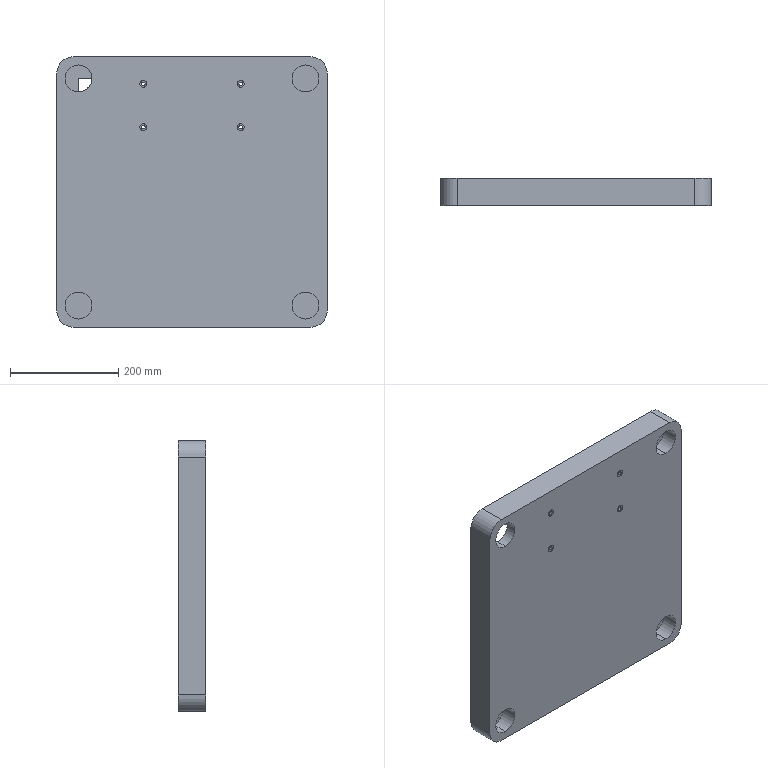Part | SolidWorks | features ICE 3, Extrusion 1, HoleWzd 1 | 1 solid | 50 faces | box 500 x 50 x 500 mm | volume 7022317 mm3 | cylinder 31 | plane 19 | commonest cylinder face diameters 6.6 x8 13 x8 50 x8 60 x4 70 x3
STEP:
#1=CARTESIAN_POINT('',(-90.,0.5,206.5));
#2=VERTEX_POINT('',#1);
#3=CARTESIAN_POINT('',(-90.,0.5,193.5));
#4=VERTEX_POINT('',#3);
#5=CARTESIAN_POINT('',(-90.,0.5,200.));
#6=DIRECTION('',(0.,-1.,0.));
#7=DIRECTION('',(0.,0.,-1.));
#8=AXIS2_PLACEMENT_3D('',#5,#6,#7);
#9=CIRCLE('',#8,6.5);
#10=EDGE_CURVE('',#2,#4,#9,.T.);
#11=ORIENTED_EDGE('',*,*,#10,.F.);
#12=CARTESIAN_POINT('',(-90.,0.,206.5));
#13=VERTEX_POINT('',#12);
#14=CARTESIAN_POINT('',(-90.,0.,206.5));
#15=DIRECTION('',(0.,-1.,0.));
#16=VECTOR('',#15,1000.);
#17=LINE('',#14,#16);
#18=EDGE_CURVE('',#2,#13,#17,.T.);
#19=ORIENTED_EDGE('',*,*,#18,.T.);
#20=CARTESIAN_POINT('',(-90.,0.,193.5));
#21=VERTEX_POINT('',#20);
#22=CARTESIAN_POINT('',(-90.,0.,200.));
#23=DIRECTION('',(0.,-1.,0.));
#24=DIRECTION('',(0.,0.,-1.));
#25=AXIS2_PLACEMENT_3D('',#22,#23,#24);
#26=CIRCLE('',#25,6.5);
#27=EDGE_CURVE('',#13,#21,#26,.T.);
#28=ORIENTED_EDGE('',*,*,#27,.T.);
#29=CARTESIAN_POINT('',(-90.,0.,193.5));
#30=DIRECTION('',(0.,-1.,0.));
#31=VECTOR('',#30,1000.);
#32=LINE('',#29,#31);
#33=EDGE_CURVE('',#4,#21,#32,.T.);
#34=ORIENTED_EDGE('',*,*,#33,.F.);
#35=EDGE_LOOP('',(#11,#19,#28,#34));
#36=FACE_OUTER_BOUND('',#35,.T.);
#37=CARTESIAN_POINT('',(-90.,0.,200.));
#38=DIRECTION('',(0.,-1.,0.));
#39=DIRECTION('',(0.,0.,-1.));
#40=AXIS2_PLACEMENT_3D('',#37,#38,#39);
#41=CYLINDRICAL_SURFACE('',#40,6.5);
#42=ADVANCED_FACE('',(#36),#41,.F.);
#43=CARTESIAN_POINT('',(-90.,20.,203.3));
#44=VERTEX_POINT('',#43);
#45=CARTESIAN_POINT('',(-90.,20.,196.7));
#46=VERTEX_POINT('',#45);
#47=CARTESIAN_POINT('',(-90.,20.,200.));
#48=DIRECTION('',(0.,-1.,0.));
#49=DIRECTION('',(0.,0.,-1.));
#50=AXIS2_PLACEMENT_3D('',#47,#48,#49);
#51=CIRCLE('',#50,3.3);
#52=EDGE_CURVE('',#44,#46,#51,.T.);
#53=ORIENTED_EDGE('',*,*,#52,.F.);
#54=CARTESIAN_POINT('',(-90.,0.5,203.3));
#55=VERTEX_POINT('',#54);
#56=CARTESIAN_POINT('',(-90.,0.,203.3));
#57=DIRECTION('',(0.,-1.,0.));
#58=VECTOR('',#57,1000.);
#59=LINE('',#56,#58);
#60=EDGE_CURVE('',#44,#55,#59,.T.);
#61=ORIENTED_EDGE('',*,*,#60,.T.);
#62=CARTESIAN_POINT('',(-90.,0.5,196.7));
#63=VERTEX_POINT('',#62);
#64=CARTESIAN_POINT('',(-90.,0.5,200.));
#65=DIRECTION('',(0.,-1.,0.));
#66=DIRECTION('',(0.,0.,-1.));
#67=AXIS2_PLACEMENT_3D('',#64,#65,#66);
#68=CIRCLE('',#67,3.3);
#69=EDGE_CURVE('',#55,#63,#68,.T.);
#70=ORIENTED_EDGE('',*,*,#69,.T.);
#71=CARTESIAN_POINT('',(-90.,0.,196.7));
#72=DIRECTION('',(0.,-1.,0.));
#73=VECTOR('',#72,1000.);
#74=LINE('',#71,#73);
#75=EDGE_CURVE('',#46,#63,#74,.T.);
#76=ORIENTED_EDGE('',*,*,#75,.F.);
#77=EDGE_LOOP('',(#53,#61,#70,#76));
#78=FACE_OUTER_BOUND('',#77,.T.);
#79=CARTESIAN_POINT('',(-90.,0.,200.));
#80=DIRECTION('',(0.,-1.,0.));
#81=DIRECTION('',(0.,0.,-1.));
#82=AXIS2_PLACEMENT_3D('',#79,#80,#81);
#83=CYLINDRICAL_SURFACE('',#82,3.3);
#84=ADVANCED_FACE('',(#78),#83,.F.);
#85=CARTESIAN_POINT('',(90.,0.5,126.5));
#86=VERTEX_POINT('',#85);
#87=CARTESIAN_POINT('',(90.,0.5,113.5));
#88=VERTEX_POINT('',#87);
#89=CARTESIAN_POINT('',(90.,0.5,120.));
#90=DIRECTION('',(0.,-1.,0.));
#91=DIRECTION('',(0.,0.,-1.));
#92=AXIS2_PLACEMENT_3D('',#89,#90,#91);
#93=CIRCLE('',#92,6.5);
#94=EDGE_CURVE('',#86,#88,#93,.T.);
#95=ORIENTED_EDGE('',*,*,#94,.F.);
#96=CARTESIAN_POINT('',(90.,0.,126.5));
#97=VERTEX_POINT('',#96);
#98=CARTESIAN_POINT('',(90.,0.,126.5));
#99=DIRECTION('',(0.,-1.,0.));
#100=VECTOR('',#99,1000.);
#101=LINE('',#98,#100);
#102=EDGE_CURVE('',#86,#97,#101,.T.);
#103=ORIENTED_EDGE('',*,*,#102,.T.);
#104=CARTESIAN_POINT('',(90.,0.,113.5));
#105=VERTEX_POINT('',#104);
#106=CARTESIAN_POINT('',(90.,0.,120.));
#107=DIRECTION('',(0.,-1.,0.));
#108=DIRECTION('',(0.,0.,-1.));
#109=AXIS2_PLACEMENT_3D('',#106,#107,#108);
#110=CIRCLE('',#109,6.5);
#111=EDGE_CURVE('',#97,#105,#110,.T.);
#112=ORIENTED_EDGE('',*,*,#111,.T.);
#113=CARTESIAN_POINT('',(90.,0.,113.5));
#114=DIRECTION('',(0.,-1.,0.));
#115=VECTOR('',#114,1000.);
#116=LINE('',#113,#115);
#117=EDGE_CURVE('',#88,#105,#116,.T.);
#118=ORIENTED_EDGE('',*,*,#117,.F.);
#119=EDGE_LOOP('',(#95,#103,#112,#118));
#120=FACE_OUTER_BOUND('',#119,.T.);
#121=CARTESIAN_POINT('',(90.,0.,120.));
#122=DIRECTION('',(0.,-1.,0.));
#123=DIRECTION('',(0.,0.,-1.));
#124=AXIS2_PLACEMENT_3D('',#121,#122,#123);
#125=CYLINDRICAL_SURFACE('',#124,6.5);
#126=ADVANCED_FACE('',(#120),#125,.F.);
#127=CARTESIAN_POINT('',(90.,20.,123.3));
#128=VERTEX_POINT('',#127);
#129=CARTESIAN_POINT('',(90.,20.,116.7));
#130=VERTEX_POINT('',#129);
#131=CARTESIAN_POINT('',(90.,20.,120.));
#132=DIRECTION('',(0.,-1.,0.));
#133=DIRECTION('',(0.,0.,-1.));
#134=AXIS2_PLACEMENT_3D('',#131,#132,#133);
#135=CIRCLE('',#134,3.3);
#136=EDGE_CURVE('',#128,#130,#135,.T.);
#137=ORIENTED_EDGE('',*,*,#136,.F.);
#138=CARTESIAN_POINT('',(90.,0.5,123.3));
#139=VERTEX_POINT('',#138);
#140=CARTESIAN_POINT('',(90.,0.,123.3));
#141=DIRECTION('',(0.,-1.,0.));
#142=VECTOR('',#141,1000.);
#143=LINE('',#140,#142);
#144=EDGE_CURVE('',#128,#139,#143,.T.);
#145=ORIENTED_EDGE('',*,*,#144,.T.);
#146=CARTESIAN_POINT('',(90.,0.5,116.7));
#147=VERTEX_POINT('',#146);
#148=CARTESIAN_POINT('',(90.,0.5,120.));
#149=DIRECTION('',(0.,-1.,0.));
#150=DIRECTION('',(0.,0.,-1.));
#151=AXIS2_PLACEMENT_3D('',#148,#149,#150);
#152=CIRCLE('',#151,3.3);
#153=EDGE_CURVE('',#139,#147,#152,.T.);
#154=ORIENTED_EDGE('',*,*,#153,.T.);
#155=CARTESIAN_POINT('',(90.,0.,116.7));
#156=DIRECTION('',(0.,-1.,0.));
#157=VECTOR('',#156,1000.);
#158=LINE('',#155,#157);
#159=EDGE_CURVE('',#130,#147,#158,.T.);
#160=ORIENTED_EDGE('',*,*,#159,.F.);
#161=EDGE_LOOP('',(#137,#145,#154,#160));
#162=FACE_OUTER_BOUND('',#161,.T.);
#163=CARTESIAN_POINT('',(90.,0.,120.));
#164=DIRECTION('',(0.,-1.,0.));
#165=DIRECTION('',(0.,0.,-1.));
#166=AXIS2_PLACEMENT_3D('',#163,#164,#165);
#167=CYLINDRICAL_SURFACE('',#166,3.3);
#168=ADVANCED_FACE('',(#162),#167,.F.);
#169=CARTESIAN_POINT('',(-90.,0.5,126.5));
#170=VERTEX_POINT('',#169);
#171=CARTESIAN_POINT('',(-90.,0.5,113.5));
#172=VERTEX_POINT('',#171);
#173=CARTESIAN_POINT('',(-90.,0.5,120.));
#174=DIRECTION('',(0.,-1.,0.));
#175=DIRECTION('',(0.,0.,-1.));
#176=AXIS2_PLACEMENT_3D('',#173,#174,#175);
#177=CIRCLE('',#176,6.5);
#178=EDGE_CURVE('',#170,#172,#177,.T.);
#179=ORIENTED_EDGE('',*,*,#178,.F.);
#180=CARTESIAN_POINT('',(-90.,0.,126.5));
#181=VERTEX_POINT('',#180);
#182=CARTESIAN_POINT('',(-90.,0.,126.5));
#183=DIRECTION('',(0.,-1.,0.));
#184=VECTOR('',#183,1000.);
#185=LINE('',#182,#184);
#186=EDGE_CURVE('',#170,#181,#185,.T.);
#187=ORIENTED_EDGE('',*,*,#186,.T.);
#188=CARTESIAN_POINT('',(-90.,0.,113.5));
#189=VERTEX_POINT('',#188);
#190=CARTESIAN_POINT('',(-90.,0.,120.));
#191=DIRECTION('',(0.,-1.,0.));
#192=DIRECTION('',(0.,0.,-1.));
#193=AXIS2_PLACEMENT_3D('',#190,#191,#192);
#194=CIRCLE('',#193,6.5);
#195=EDGE_CURVE('',#181,#189,#194,.T.);
#196=ORIENTED_EDGE('',*,*,#195,.T.);
#197=CARTESIAN_POINT('',(-90.,0.,113.5));
#198=DIRECTION('',(0.,-1.,0.));
#199=VECTOR('',#198,1000.);
#200=LINE('',#197,#199);
#201=EDGE_CURVE('',#172,#189,#200,.T.);
#202=ORIENTED_EDGE('',*,*,#201,.F.);
#203=EDGE_LOOP('',(#179,#187,#196,#202));
#204=FACE_OUTER_BOUND('',#203,.T.);
#205=CARTESIAN_POINT('',(-90.,0.,120.));
#206=DIRECTION('',(0.,-1.,0.));
#207=DIRECTION('',(0.,0.,-1.));
#208=AXIS2_PLACEMENT_3D('',#205,#206,#207);
#209=CYLINDRICAL_SURFACE('',#208,6.5);
#210=ADVANCED_FACE('',(#204),#209,.F.);
#211=CARTESIAN_POINT('',(-90.,20.,123.3));
#212=VERTEX_POINT('',#211);
#213=CARTESIAN_POINT('',(-90.,20.,116.7));
#214=VERTEX_POINT('',#213);
#215=CARTESIAN_POINT('',(-90.,20.,120.));
#216=DIRECTION('',(0.,-1.,0.));
#217=DIRECTION('',(0.,0.,-1.));
#218=AXIS2_PLACEMENT_3D('',#215,#216,#217);
#219=CIRCLE('',#218,3.3);
#220=EDGE_CURVE('',#212,#214,#219,.T.);
#221=ORIENTED_EDGE('',*,*,#220,.F.);
#222=CARTESIAN_POINT('',(-90.,0.5,123.3));
#223=VERTEX_POINT('',#222);
#224=CARTESIAN_POINT('',(-90.,0.,123.3));
#225=DIRECTION('',(0.,-1.,0.));
#226=VECTOR('',#225,1000.);
#227=LINE('',#224,#226);
#228=EDGE_CURVE('',#212,#223,#227,.T.);
#229=ORIENTED_EDGE('',*,*,#228,.T.);
#230=CARTESIAN_POINT('',(-90.,0.5,116.7));
#231=VERTEX_POINT('',#230);
#232=CARTESIAN_POINT('',(-90.,0.5,120.));
#233=DIRECTION('',(0.,-1.,0.));
#234=DIRECTION('',(0.,0.,-1.));
#235=AXIS2_PLACEMENT_3D('',#232,#233,#234);
#236=CIRCLE('',#235,3.3);
#237=EDGE_CURVE('',#223,#231,#236,.T.);
#238=ORIENTED_EDGE('',*,*,#237,.T.);
#239=CARTESIAN_POINT('',(-90.,0.,116.7));
#240=DIRECTION('',(0.,-1.,0.));
#241=VECTOR('',#240,1000.);
#242=LINE('',#239,#241);
#243=EDGE_CURVE('',#214,#231,#242,.T.);
#244=ORIENTED_EDGE('',*,*,#243,.F.);
#245=EDGE_LOOP('',(#221,#229,#238,#244));
#246=FACE_OUTER_BOUND('',#245,.T.);
#247=CARTESIAN_POINT('',(-90.,0.,120.));
#248=DIRECTION('',(0.,-1.,0.));
#249=DIRECTION('',(0.,0.,-1.));
#250=AXIS2_PLACEMENT_3D('',#247,#248,#249);
#251=CYLINDRICAL_SURFACE('',#250,3.3);
#252=ADVANCED_FACE('',(#246),#251,.F.);
#253=CARTESIAN_POINT('',(90.,0.5,206.5));
#254=VERTEX_POINT('',#253);
#255=CARTESIAN_POINT('',(90.,0.5,193.5));
#256=VERTEX_POINT('',#255);
#257=CARTESIAN_POINT('',(90.,0.5,200.));
#258=DIRECTION('',(0.,-1.,0.));
#259=DIRECTION('',(0.,0.,-1.));
#260=AXIS2_PLACEMENT_3D('',#257,#258,#259);
#261=CIRCLE('',#260,6.5);
#262=EDGE_CURVE('',#254,#256,#261,.T.);
#263=ORIENTED_EDGE('',*,*,#262,.F.);
#264=CARTESIAN_POINT('',(90.,0.,206.5));
#265=VERTEX_POINT('',#264);
#266=CARTESIAN_POINT('',(90.,0.,206.5));
#267=DIRECTION('',(0.,-1.,0.));
#268=VECTOR('',#267,1000.);
#269=LINE('',#266,#268);
#270=EDGE_CURVE('',#254,#265,#269,.T.);
#271=ORIENTED_EDGE('',*,*,#270,.T.);
#272=CARTESIAN_POINT('',(90.,0.,193.5));
#273=VERTEX_POINT('',#272);
#274=CARTESIAN_POINT('',(90.,0.,200.));
#275=DIRECTION('',(0.,-1.,0.));
#276=DIRECTION('',(0.,0.,-1.));
#277=AXIS2_PLACEMENT_3D('',#274,#275,#276);
#278=CIRCLE('',#277,6.5);
#279=EDGE_CURVE('',#265,#273,#278,.T.);
#280=ORIENTED_EDGE('',*,*,#279,.T.);
#281=CARTESIAN_POINT('',(90.,0.,193.5));
#282=DIRECTION('',(0.,-1.,0.));
#283=VECTOR('',#282,1000.);
#284=LINE('',#281,#283);
#285=EDGE_CURVE('',#256,#273,#284,.T.);
#286=ORIENTED_EDGE('',*,*,#285,.F.);
#287=EDGE_LOOP('',(#263,#271,#280,#286));
#288=FACE_OUTER_BOUND('',#287,.T.);
#289=CARTESIAN_POINT('',(90.,0.,200.));
#290=DIRECTION('',(0.,-1.,0.));
#291=DIRECTION('',(0.,0.,-1.));
#292=AXIS2_PLACEMENT_3D('',#289,#290,#291);
#293=CYLINDRICAL_SURFACE('',#292,6.5);
#294=ADVANCED_FACE('',(#288),#293,.F.);
#295=CARTESIAN_POINT('',(90.,20.,203.3));
#296=VERTEX_POINT('',#295);
#297=CARTESIAN_POINT('',(90.,20.,196.7));
#298=VERTEX_POINT('',#297);
#299=CARTESIAN_POINT('',(90.,20.,200.));
#300=DIRECTION('',(0.,-1.,0.));
#301=DIRECTION('',(0.,0.,-1.));
#302=AXIS2_PLACEMENT_3D('',#299,#300,#301);
#303=CIRCLE('',#302,3.3);
#304=EDGE_CURVE('',#296,#298,#303,.T.);
#305=ORIENTED_EDGE('',*,*,#304,.F.);
#306=CARTESIAN_POINT('',(90.,0.5,203.3));
#307=VERTEX_POINT('',#306);
#308=CARTESIAN_POINT('',(90.,0.,203.3));
#309=DIRECTION('',(0.,-1.,0.));
#310=VECTOR('',#309,1000.);
#311=LINE('',#308,#310);
#312=EDGE_CURVE('',#296,#307,#311,.T.);
#313=ORIENTED_EDGE('',*,*,#312,.T.);
#314=CARTESIAN_POINT('',(90.,0.5,196.7));
#315=VERTEX_POINT('',#314);
#316=CARTESIAN_POINT('',(90.,0.5,200.));
#317=DIRECTION('',(0.,-1.,0.));
#318=DIRECTION('',(0.,0.,-1.));
#319=AXIS2_PLACEMENT_3D('',#316,#317,#318);
#320=CIRCLE('',#319,3.3);
#321=EDGE_CURVE('',#307,#315,#320,.T.);
#322=ORIENTED_EDGE('',*,*,#321,.T.);
#323=CARTESIAN_POINT('',(90.,0.,196.7));
#324=DIRECTION('',(0.,-1.,0.));
#325=VECTOR('',#324,1000.);
#326=LINE('',#323,#325);
#327=EDGE_CURVE('',#298,#315,#326,.T.);
#328=ORIENTED_EDGE('',*,*,#327,.F.);
#329=EDGE_LOOP('',(#305,#313,#322,#328));
#330=FACE_OUTER_BOUND('',#329,.T.);
#331=CARTESIAN_POINT('',(90.,0.,200.));
#332=DIRECTION('',(0.,-1.,0.));
#333=DIRECTION('',(0.,0.,-1.));
#334=AXIS2_PLACEMENT_3D('',#331,#332,#333);
#335=CYLINDRICAL_SURFACE('',#334,3.3);
#336=ADVANCED_FACE('',(#330),#335,.F.);
#337=CARTESIAN_POINT('',(-210.,30.,-185.));
#338=VERTEX_POINT('',#337);
#339=CARTESIAN_POINT('',(-210.,30.,-235.));
#340=VERTEX_POINT('',#339);
#341=CARTESIAN_POINT('',(-210.,30.,-210.));
#342=DIRECTION('',(0.,-1.,0.));
#343=DIRECTION('',(0.,0.,1.));
#344=AXIS2_PLACEMENT_3D('',#341,#342,#343);
#345=CIRCLE('',#344,25.);
#346=EDGE_CURVE('',#338,#340,#345,.T.);
#347=ORIENTED_EDGE('',*,*,#346,.F.);
#348=CARTESIAN_POINT('',(-210.,0.,-185.));
#349=VERTEX_POINT('',#348);
#350=CARTESIAN_POINT('',(-210.,30.,-185.));
#351=DIRECTION('',(0.,-1.,0.));
#352=VECTOR('',#351,1000.);
#353=LINE('',#350,#352);
#354=EDGE_CURVE('',#338,#349,#353,.T.);
#355=ORIENTED_EDGE('',*,*,#354,.T.);
#356=CARTESIAN_POINT('',(-210.,0.,-235.));
#357=VERTEX_POINT('',#356);
#358=CARTESIAN_POINT('',(-210.,0.,-210.));
#359=DIRECTION('',(0.,-1.,0.));
#360=DIRECTION('',(0.,0.,1.));
#361=AXIS2_PLACEMENT_3D('',#358,#359,#360);
#362=CIRCLE('',#361,25.);
#363=EDGE_CURVE('',#349,#357,#362,.T.);
#364=ORIENTED_EDGE('',*,*,#363,.T.);
#365=CARTESIAN_POINT('',(-210.,30.,-235.));
#366=DIRECTION('',(0.,-1.,0.));
#367=VECTOR('',#366,1000.);
#368=LINE('',#365,#367);
#369=EDGE_CURVE('',#340,#357,#368,.T.);
#370=ORIENTED_EDGE('',*,*,#369,.F.);
#371=EDGE_LOOP('',(#347,#355,#364,#370));
#372=FACE_OUTER_BOUND('',#371,.T.);
#373=CARTESIAN_POINT('',(-210.,30.,-210.));
#374=DIRECTION('',(0.,-1.,0.));
#375=DIRECTION('',(0.,0.,-1.));
#376=AXIS2_PLACEMENT_3D('',#373,#374,#375);
#377=CYLINDRICAL_SURFACE('',#376,25.);
#378=ADVANCED_FACE('',(#372),#377,.F.);
#379=CARTESIAN_POINT('',(210.,30.,-185.));
#380=VERTEX_POINT('',#379);
#381=CARTESIAN_POINT('',(210.,30.,-235.));
#382=VERTEX_POINT('',#381);
#383=CARTESIAN_POINT('',(210.,30.,-210.));
#384=DIRECTION('',(0.,-1.,0.));
#385=DIRECTION('',(0.,0.,-1.));
#386=AXIS2_PLACEMENT_3D('',#383,#384,#385);
#387=CIRCLE('',#386,25.);
#388=EDGE_CURVE('',#380,#382,#387,.T.);
#389=ORIENTED_EDGE('',*,*,#388,.F.);
#390=CARTESIAN_POINT('',(210.,0.,-185.));
#391=VERTEX_POINT('',#390);
#392=CARTESIAN_POINT('',(210.,30.,-185.));
#393=DIRECTION('',(0.,-1.,0.));
#394=VECTOR('',#393,1000.);
#395=LINE('',#392,#394);
#396=EDGE_CURVE('',#380,#391,#395,.T.);
#397=ORIENTED_EDGE('',*,*,#396,.T.);
#398=CARTESIAN_POINT('',(210.,0.,-235.));
#399=VERTEX_POINT('',#398);
#400=CARTESIAN_POINT('',(210.,0.,-210.));
#401=DIRECTION('',(0.,-1.,0.));
#402=DIRECTION('',(0.,0.,-1.));
#403=AXIS2_PLACEMENT_3D('',#400,#401,#402);
#404=CIRCLE('',#403,25.);
#405=EDGE_CURVE('',#391,#399,#404,.T.);
#406=ORIENTED_EDGE('',*,*,#405,.T.);
#407=CARTESIAN_POINT('',(210.,30.,-235.));
#408=DIRECTION('',(0.,-1.,0.));
#409=VECTOR('',#408,1000.);
#410=LINE('',#407,#409);
#411=EDGE_CURVE('',#382,#399,#410,.T.);
#412=ORIENTED_EDGE('',*,*,#411,.F.);
#413=EDGE_LOOP('',(#389,#397,#406,#412));
#414=FACE_OUTER_BOUND('',#413,.T.);
#415=CARTESIAN_POINT('',(210.,30.,-210.));
#416=DIRECTION('',(0.,-1.,0.));
#417=DIRECTION('',(0.,0.,-1.));
#418=AXIS2_PLACEMENT_3D('',#415,#416,#417);
#419=CYLINDRICAL_SURFACE('',#418,25.);
#420=ADVANCED_FACE('',(#414),#419,.F.);
#421=CARTESIAN_POINT('',(210.,30.,235.));
#422=VERTEX_POINT('',#421);
#423=CARTESIAN_POINT('',(210.,30.,185.));
#424=VERTEX_POINT('',#423);
#425=CARTESIAN_POINT('',(210.,30.,210.));
#426=DIRECTION('',(0.,-1.,0.));
#427=DIRECTION('',(0.,0.,1.));
#428=AXIS2_PLACEMENT_3D('',#425,#426,#427);
#429=CIRCLE('',#428,25.);
#430=EDGE_CURVE('',#422,#424,#429,.T.);
#431=ORIENTED_EDGE('',*,*,#430,.F.);
#432=CARTESIAN_POINT('',(210.,0.,235.));
#433=VERTEX_POINT('',#432);
#434=CARTESIAN_POINT('',(210.,30.,235.));
#435=DIRECTION('',(0.,-1.,0.));
#436=VECTOR('',#435,1000.);
#437=LINE('',#434,#436);
#438=EDGE_CURVE('',#422,#433,#437,.T.);
#439=ORIENTED_EDGE('',*,*,#438,.T.);
#440=CARTESIAN_POINT('',(210.,0.,185.));
#441=VERTEX_POINT('',#440);
#442=CARTESIAN_POINT('',(210.,0.,210.));
#443=DIRECTION('',(0.,-1.,0.));
#444=DIRECTION('',(0.,0.,1.));
#445=AXIS2_PLACEMENT_3D('',#442,#443,#444);
#446=CIRCLE('',#445,25.);
#447=EDGE_CURVE('',#433,#441,#446,.T.);
#448=ORIENTED_EDGE('',*,*,#447,.T.);
#449=CARTESIAN_POINT('',(210.,30.,185.));
#450=DIRECTION('',(0.,-1.,0.));
#451=VECTOR('',#450,1000.);
#452=LINE('',#449,#451);
#453=EDGE_CURVE('',#424,#441,#452,.T.);
#454=ORIENTED_EDGE('',*,*,#453,.F.);
#455=EDGE_LOOP('',(#431,#439,#448,#454));
#456=FACE_OUTER_BOUND('',#455,.T.);
#457=CARTESIAN_POINT('',(210.,30.,210.));
#458=DIRECTION('',(0.,-1.,0.));
#459=DIRECTION('',(0.,0.,-1.));
#460=AXIS2_PLACEMENT_3D('',#457,#458,#459);
#461=CYLINDRICAL_SURFACE('',#460,25.);
#462=ADVANCED_FACE('',(#456),#461,.F.);
#463=CARTESIAN_POINT('',(-210.,30.,235.));
#464=VERTEX_POINT('',#463);
#465=CARTESIAN_POINT('',(-210.,30.,185.));
#466=VERTEX_POINT('',#465);
#467=CARTESIAN_POINT('',(-210.,30.,210.));
#468=DIRECTION('',(0.,-1.,0.));
#469=DIRECTION('',(0.,0.,-1.));
#470=AXIS2_PLACEMENT_3D('',#467,#468,#469);
#471=CIRCLE('',#470,25.);
#472=EDGE_CURVE('',#464,#466,#471,.T.);
#473=ORIENTED_EDGE('',*,*,#472,.F.);
#474=CARTESIAN_POINT('',(-210.,0.,235.));
#475=VERTEX_POINT('',#474);
#476=CARTESIAN_POINT('',(-210.,30.,235.));
#477=DIRECTION('',(0.,-1.,0.));
#478=VECTOR('',#477,1000.);
#479=LINE('',#476,#478);
#480=EDGE_CURVE('',#464,#475,#479,.T.);
#481=ORIENTED_EDGE('',*,*,#480,.T.);
#482=CARTESIAN_POINT('',(-210.,0.,185.));
#483=VERTEX_POINT('',#482);
#484=CARTESIAN_POINT('',(-210.,0.,210.));
#485=DIRECTION('',(0.,-1.,0.));
#486=DIRECTION('',(0.,0.,-1.));
#487=AXIS2_PLACEMENT_3D('',#484,#485,#486);
#488=CIRCLE('',#487,25.);
#489=EDGE_CURVE('',#475,#483,#488,.T.);
#490=ORIENTED_EDGE('',*,*,#489,.T.);
#491=CARTESIAN_POINT('',(-210.,20.,185.));
#492=VERTEX_POINT('',#491);
#493=CARTESIAN_POINT('',(-210.,30.,185.));
#494=DIRECTION('',(0.,-1.,0.));
#495=VECTOR('',#494,1000.);
#496=LINE('',#493,#495);
#497=EDGE_CURVE('',#492,#483,#496,.T.);
#498=ORIENTED_EDGE('',*,*,#497,.F.);
#499=CARTESIAN_POINT('',(-210.,30.,185.));
#500=DIRECTION('',(0.,1.,0.));
#501=VECTOR('',#500,1000.);
#502=LINE('',#499,#501);
#503=EDGE_CURVE('',#492,#466,#502,.T.);
#504=ORIENTED_EDGE('',*,*,#503,.T.);
#505=EDGE_LOOP('',(#473,#481,#490,#498,#504));
#506=FACE_OUTER_BOUND('',#505,.T.);
#507=CARTESIAN_POINT('',(-210.,30.,210.));
#508=DIRECTION('',(0.,-1.,0.));
#509=DIRECTION('',(0.,0.,-1.));
#510=AXIS2_PLACEMENT_3D('',#507,#508,#509);
#511=CYLINDRICAL_SURFACE('',#510,25.);
#512=ADVANCED_FACE('',(#506),#511,.F.);
#513=CARTESIAN_POINT('',(-250.,0.,220.));
#514=VERTEX_POINT('',#513);
#515=CARTESIAN_POINT('',(-220.,0.,250.));
#516=VERTEX_POINT('',#515);
#517=CARTESIAN_POINT('',(-220.,0.,220.));
#518=DIRECTION('',(0.,1.,0.));
#519=DIRECTION('',(0.,0.,-1.));
#520=AXIS2_PLACEMENT_3D('',#517,#518,#519);
#521=CIRCLE('',#520,30.);
#522=EDGE_CURVE('',#514,#516,#521,.T.);
#523=ORIENTED_EDGE('',*,*,#522,.T.);
#524=CARTESIAN_POINT('',(-220.,50.,250.));
#525=VERTEX_POINT('',#524);
#526=CARTESIAN_POINT('',(-220.,50.,250.));
#527=DIRECTION('',(0.,-1.,0.));
#528=VECTOR('',#527,1000.);
#529=LINE('',#526,#528);
#530=EDGE_CURVE('',#525,#516,#529,.T.);
#531=ORIENTED_EDGE('',*,*,#530,.F.);
#532=CARTESIAN_POINT('',(-250.,50.,220.));
#533=VERTEX_POINT('',#532);
#534=CARTESIAN_POINT('',(-220.,50.,220.));
#535=DIRECTION('',(0.,1.,0.));
#536=DIRECTION('',(0.,0.,-1.));
#537=AXIS2_PLACEMENT_3D('',#534,#535,#536);
#538=CIRCLE('',#537,30.);
#539=EDGE_CURVE('',#533,#525,#538,.T.);
#540=ORIENTED_EDGE('',*,*,#539,.F.);
#541=CARTESIAN_POINT('',(-250.,50.,220.));
#542=DIRECTION('',(0.,-1.,0.));
#543=VECTOR('',#542,1000.);
#544=LINE('',#541,#543);
#545=EDGE_CURVE('',#533,#514,#544,.T.);
#546=ORIENTED_EDGE('',*,*,#545,.T.);
#547=EDGE_LOOP('',(#523,#531,#540,#546));
#548=FACE_OUTER_BOUND('',#547,.T.);
#549=CARTESIAN_POINT('',(-220.,50.,220.));
#550=DIRECTION('',(0.,-1.,0.));
#551=DIRECTION('',(0.,0.,-1.));
#552=AXIS2_PLACEMENT_3D('',#549,#550,#551);
#553=CYLINDRICAL_SURFACE('',#552,30.);
#554=ADVANCED_FACE('',(#548),#553,.T.);
#555=CARTESIAN_POINT('',(220.,0.,250.));
#556=VERTEX_POINT('',#555);
#557=CARTESIAN_POINT('',(-220.,0.,250.));
#558=DIRECTION('',(1.,0.,0.));
#559=VECTOR('',#558,1000.);
#560=LINE('',#557,#559);
#561=EDGE_CURVE('',#516,#556,#560,.T.);
#562=ORIENTED_EDGE('',*,*,#561,.T.);
#563=CARTESIAN_POINT('',(220.,50.,250.));
#564=VERTEX_POINT('',#563);
#565=CARTESIAN_POINT('',(220.,50.,250.));
#566=DIRECTION('',(0.,-1.,0.));
#567=VECTOR('',#566,1000.);
#568=LINE('',#565,#567);
#569=EDGE_CURVE('',#564,#556,#568,.T.);
#570=ORIENTED_EDGE('',*,*,#569,.F.);
#571=CARTESIAN_POINT('',(-220.,50.,250.));
#572=DIRECTION('',(1.,0.,0.));
#573=VECTOR('',#572,1000.);
#574=LINE('',#571,#573);
#575=EDGE_CURVE('',#525,#564,#574,.T.);
#576=ORIENTED_EDGE('',*,*,#575,.F.);
#577=ORIENTED_EDGE('',*,*,#530,.T.);
#578=EDGE_LOOP('',(#562,#570,#576,#577));
#579=FACE_OUTER_BOUND('',#578,.T.);
#580=CARTESIAN_POINT('',(-220.,50.,250.));
#581=DIRECTION('',(0.,0.,-1.));
#582=DIRECTION('',(-1.,0.,0.));
#583=AXIS2_PLACEMENT_3D('',#580,#581,#582);
#584=PLANE('',#583);
#585=ADVANCED_FACE('',(#579),#584,.F.);
#586=CARTESIAN_POINT('',(250.,0.,220.));
#587=VERTEX_POINT('',#586);
#588=CARTESIAN_POINT('',(220.,0.,220.));
#589=DIRECTION('',(0.,1.,0.));
#590=DIRECTION('',(0.,0.,1.));
#591=AXIS2_PLACEMENT_3D('',#588,#589,#590);
#592=CIRCLE('',#591,30.);
#593=EDGE_CURVE('',#556,#587,#592,.T.);
#594=ORIENTED_EDGE('',*,*,#593,.T.);
#595=CARTESIAN_POINT('',(250.,50.,220.));
#596=VERTEX_POINT('',#595);
#597=CARTESIAN_POINT('',(250.,50.,220.));
#598=DIRECTION('',(0.,-1.,0.));
#599=VECTOR('',#598,1000.);
#600=LINE('',#597,#599);
#601=EDGE_CURVE('',#596,#587,#600,.T.);
#602=ORIENTED_EDGE('',*,*,#601,.F.);
#603=CARTESIAN_POINT('',(220.,50.,220.));
#604=DIRECTION('',(0.,1.,0.));
#605=DIRECTION('',(0.,0.,1.));
#606=AXIS2_PLACEMENT_3D('',#603,#604,#605);
#607=CIRCLE('',#606,30.);
#608=EDGE_CURVE('',#564,#596,#607,.T.);
#609=ORIENTED_EDGE('',*,*,#608,.F.);
#610=ORIENTED_EDGE('',*,*,#569,.T.);
#611=EDGE_LOOP('',(#594,#602,#609,#610));
#612=FACE_OUTER_BOUND('',#611,.T.);
#613=CARTESIAN_POINT('',(220.,50.,220.));
#614=DIRECTION('',(0.,-1.,0.));
#615=DIRECTION('',(0.,0.,-1.));
#616=AXIS2_PLACEMENT_3D('',#613,#614,#615);
#617=CYLINDRICAL_SURFACE('',#616,30.);
#618=ADVANCED_FACE('',(#612),#617,.T.);
#619=CARTESIAN_POINT('',(250.,0.,-220.));
#620=VERTEX_POINT('',#619);
#621=CARTESIAN_POINT('',(250.,0.,220.));
#622=DIRECTION('',(0.,0.,-1.));
#623=VECTOR('',#622,1000.);
#624=LINE('',#621,#623);
#625=EDGE_CURVE('',#587,#620,#624,.T.);
#626=ORIENTED_EDGE('',*,*,#625,.T.);
#627=CARTESIAN_POINT('',(250.,50.,-220.));
#628=VERTEX_POINT('',#627);
#629=CARTESIAN_POINT('',(250.,50.,-220.));
#630=DIRECTION('',(0.,-1.,0.));
#631=VECTOR('',#630,1000.);
#632=LINE('',#629,#631);
#633=EDGE_CURVE('',#628,#620,#632,.T.);
#634=ORIENTED_EDGE('',*,*,#633,.F.);
#635=CARTESIAN_POINT('',(250.,50.,220.));
#636=DIRECTION('',(0.,0.,-1.));
#637=VECTOR('',#636,1000.);
#638=LINE('',#635,#637);
#639=EDGE_CURVE('',#596,#628,#638,.T.);
#640=ORIENTED_EDGE('',*,*,#639,.F.);
#641=ORIENTED_EDGE('',*,*,#601,.T.);
#642=EDGE_LOOP('',(#626,#634,#640,#641));
#643=FACE_OUTER_BOUND('',#642,.T.);
#644=CARTESIAN_POINT('',(250.,50.,220.));
#645=DIRECTION('',(-1.,0.,0.));
#646=DIRECTION('',(0.,0.,1.));
#647=AXIS2_PLACEMENT_3D('',#644,#645,#646);
#648=PLANE('',#647);
#649=ADVANCED_FACE('',(#643),#648,.F.);
#650=CARTESIAN_POINT('',(220.,0.,-250.));
#651=VERTEX_POINT('',#650);
#652=CARTESIAN_POINT('',(220.,0.,-220.));
#653=DIRECTION('',(0.,1.,0.));
#654=DIRECTION('',(0.,0.,1.));
#655=AXIS2_PLACEMENT_3D('',#652,#653,#654);
#656=CIRCLE('',#655,30.);
#657=EDGE_CURVE('',#620,#651,#656,.T.);
#658=ORIENTED_EDGE('',*,*,#657,.T.);
#659=CARTESIAN_POINT('',(220.,50.,-250.));
#660=VERTEX_POINT('',#659);
#661=CARTESIAN_POINT('',(220.,50.,-250.));
#662=DIRECTION('',(0.,-1.,0.));
#663=VECTOR('',#662,1000.);
#664=LINE('',#661,#663);
#665=EDGE_CURVE('',#660,#651,#664,.T.);
#666=ORIENTED_EDGE('',*,*,#665,.F.);
#667=CARTESIAN_POINT('',(220.,50.,-220.));
#668=DIRECTION('',(0.,1.,0.));
#669=DIRECTION('',(0.,0.,1.));
#670=AXIS2_PLACEMENT_3D('',#667,#668,#669);
#671=CIRCLE('',#670,30.);
#672=EDGE_CURVE('',#628,#660,#671,.T.);
#673=ORIENTED_EDGE('',*,*,#672,.F.);
#674=ORIENTED_EDGE('',*,*,#633,.T.);
#675=EDGE_LOOP('',(#658,#666,#673,#674));
#676=FACE_OUTER_BOUND('',#675,.T.);
#677=CARTESIAN_POINT('',(220.,50.,-220.));
#678=DIRECTION('',(0.,-1.,0.));
#679=DIRECTION('',(0.,0.,-1.));
#680=AXIS2_PLACEMENT_3D('',#677,#678,#679);
#681=CYLINDRICAL_SURFACE('',#680,30.);
#682=ADVANCED_FACE('',(#676),#681,.T.);
#683=CARTESIAN_POINT('',(-220.,0.,-250.));
#684=VERTEX_POINT('',#683);
#685=CARTESIAN_POINT('',(-220.,0.,-250.));
#686=DIRECTION('',(-1.,0.,0.));
#687=VECTOR('',#686,1000.);
#688=LINE('',#685,#687);
#689=EDGE_CURVE('',#651,#684,#688,.T.);
#690=ORIENTED_EDGE('',*,*,#689,.T.);
#691=CARTESIAN_POINT('',(-220.,50.,-250.));
#692=VERTEX_POINT('',#691);
#693=CARTESIAN_POINT('',(-220.,50.,-250.));
#694=DIRECTION('',(0.,-1.,0.));
#695=VECTOR('',#694,1000.);
#696=LINE('',#693,#695);
#697=EDGE_CURVE('',#692,#684,#696,.T.);
#698=ORIENTED_EDGE('',*,*,#697,.F.);
#699=CARTESIAN_POINT('',(-220.,50.,-250.));
#700=DIRECTION('',(-1.,0.,0.));
#701=VECTOR('',#700,1000.);
#702=LINE('',#699,#701);
#703=EDGE_CURVE('',#660,#692,#702,.T.);
#704=ORIENTED_EDGE('',*,*,#703,.F.);
#705=ORIENTED_EDGE('',*,*,#665,.T.);
#706=EDGE_LOOP('',(#690,#698,#704,#705));
#707=FACE_OUTER_BOUND('',#706,.T.);
#708=CARTESIAN_POINT('',(-220.,50.,-250.));
#709=DIRECTION('',(0.,0.,1.));
#710=DIRECTION('',(1.,0.,0.));
#711=AXIS2_PLACEMENT_3D('',#708,#709,#710);
#712=PLANE('',#711);
#713=ADVANCED_FACE('',(#707),#712,.F.);
#714=CARTESIAN_POINT('',(-250.,0.,-220.));
#715=VERTEX_POINT('',#714);
#716=CARTESIAN_POINT('',(-220.,0.,-220.));
#717=DIRECTION('',(0.,1.,0.));
#718=DIRECTION('',(0.,0.,-1.));
#719=AXIS2_PLACEMENT_3D('',#716,#717,#718);
#720=CIRCLE('',#719,30.);
#721=EDGE_CURVE('',#684,#715,#720,.T.);
#722=ORIENTED_EDGE('',*,*,#721,.T.);
#723=CARTESIAN_POINT('',(-250.,50.,-220.));
#724=VERTEX_POINT('',#723);
#725=CARTESIAN_POINT('',(-250.,50.,-220.));
#726=DIRECTION('',(0.,-1.,0.));
#727=VECTOR('',#726,1000.);
#728=LINE('',#725,#727);
#729=EDGE_CURVE('',#724,#715,#728,.T.);
#730=ORIENTED_EDGE('',*,*,#729,.F.);
#731=CARTESIAN_POINT('',(-220.,50.,-220.));
#732=DIRECTION('',(0.,1.,0.));
#733=DIRECTION('',(0.,0.,-1.));
#734=AXIS2_PLACEMENT_3D('',#731,#732,#733);
#735=CIRCLE('',#734,30.);
#736=EDGE_CURVE('',#692,#724,#735,.T.);
#737=ORIENTED_EDGE('',*,*,#736,.F.);
#738=ORIENTED_EDGE('',*,*,#697,.T.);
#739=EDGE_LOOP('',(#722,#730,#737,#738));
#740=FACE_OUTER_BOUND('',#739,.T.);
#741=CARTESIAN_POINT('',(-220.,50.,-220.));
#742=DIRECTION('',(0.,-1.,0.));
#743=DIRECTION('',(0.,0.,-1.));
#744=AXIS2_PLACEMENT_3D('',#741,#742,#743);
#745=CYLINDRICAL_SURFACE('',#744,30.);
#746=ADVANCED_FACE('',(#740),#745,.T.);
#747=CARTESIAN_POINT('',(-250.,0.,220.));
#748=DIRECTION('',(0.,0.,1.));
#749=VECTOR('',#748,1000.);
#750=LINE('',#747,#749);
#751=EDGE_CURVE('',#715,#514,#750,.T.);
#752=ORIENTED_EDGE('',*,*,#751,.T.);
#753=ORIENTED_EDGE('',*,*,#545,.F.);
#754=CARTESIAN_POINT('',(-250.,50.,220.));
#755=DIRECTION('',(0.,0.,1.));
#756=VECTOR('',#755,1000.);
#757=LINE('',#754,#756);
#758=EDGE_CURVE('',#724,#533,#757,.T.);
#759=ORIENTED_EDGE('',*,*,#758,.F.);
#760=ORIENTED_EDGE('',*,*,#729,.T.);
#761=EDGE_LOOP('',(#752,#753,#759,#760));
#762=FACE_OUTER_BOUND('',#761,.T.);
#763=CARTESIAN_POINT('',(-250.,50.,220.));
#764=DIRECTION('',(1.,0.,0.));
#765=DIRECTION('',(0.,0.,-1.));
#766=AXIS2_PLACEMENT_3D('',#763,#764,#765);
#767=PLANE('',#766);
#768=ADVANCED_FACE('',(#762),#767,.F.);
#769=CARTESIAN_POINT('',(-210.,50.,210.));
#770=VERTEX_POINT('',#769);
#771=CARTESIAN_POINT('',(175.,50.,210.));
#772=VERTEX_POINT('',#771);
#773=CARTESIAN_POINT('',(-175.,50.,210.));
#774=DIRECTION('',(1.,0.,0.));
#775=VECTOR('',#774,1000.);
#776=LINE('',#773,#775);
#777=EDGE_CURVE('',#770,#772,#776,.T.);
#778=ORIENTED_EDGE('',*,*,#777,.F.);
#779=CARTESIAN_POINT('',(-210.,50.,-175.));
#780=VERTEX_POINT('',#779);
#781=CARTESIAN_POINT('',(-210.,50.,175.));
#782=DIRECTION('',(0.,0.,1.));
#783=VECTOR('',#782,1000.);
#784=LINE('',#781,#783);
#785=EDGE_CURVE('',#780,#770,#784,.T.);
#786=ORIENTED_EDGE('',*,*,#785,.F.);
#787=CARTESIAN_POINT('',(-175.,50.,-210.));
#788=VERTEX_POINT('',#787);
#789=CARTESIAN_POINT('',(-210.,50.,-210.));
#790=DIRECTION('',(0.,-1.,0.));
#791=DIRECTION('',(0.,0.,-1.));
#792=AXIS2_PLACEMENT_3D('',#789,#790,#791);
#793=CIRCLE('',#792,35.);
#794=EDGE_CURVE('',#788,#780,#793,.T.);
#795=ORIENTED_EDGE('',*,*,#794,.F.);
#796=CARTESIAN_POINT('',(175.,50.,-210.));
#797=VERTEX_POINT('',#796);
#798=CARTESIAN_POINT('',(-175.,50.,-210.));
#799=DIRECTION('',(-1.,0.,0.));
#800=VECTOR('',#799,1000.);
#801=LINE('',#798,#800);
#802=EDGE_CURVE('',#797,#788,#801,.T.);
#803=ORIENTED_EDGE('',*,*,#802,.F.);
#804=CARTESIAN_POINT('',(210.,50.,-175.));
#805=VERTEX_POINT('',#804);
#806=CARTESIAN_POINT('',(210.,50.,-210.));
#807=DIRECTION('',(0.,-1.,0.));
#808=DIRECTION('',(0.,0.,1.));
#809=AXIS2_PLACEMENT_3D('',#806,#807,#808);
#810=CIRCLE('',#809,35.);
#811=EDGE_CURVE('',#805,#797,#810,.T.);
#812=ORIENTED_EDGE('',*,*,#811,.F.);
#813=CARTESIAN_POINT('',(210.,50.,175.));
#814=VERTEX_POINT('',#813);
#815=CARTESIAN_POINT('',(210.,50.,175.));
#816=DIRECTION('',(0.,0.,-1.));
#817=VECTOR('',#816,1000.);
#818=LINE('',#815,#817);
#819=EDGE_CURVE('',#814,#805,#818,.T.);
#820=ORIENTED_EDGE('',*,*,#819,.F.);
#821=CARTESIAN_POINT('',(210.,50.,210.));
#822=DIRECTION('',(0.,-1.,0.));
#823=DIRECTION('',(0.,0.,-1.));
#824=AXIS2_PLACEMENT_3D('',#821,#822,#823);
#825=CIRCLE('',#824,35.);
#826=EDGE_CURVE('',#772,#814,#825,.T.);
#827=ORIENTED_EDGE('',*,*,#826,.F.);
#828=EDGE_LOOP('',(#778,#786,#795,#803,#812,#820,#827));
#829=FACE_BOUND('',#828,.T.);
#830=ORIENTED_EDGE('',*,*,#539,.T.);
#831=ORIENTED_EDGE('',*,*,#575,.T.);
#832=ORIENTED_EDGE('',*,*,#608,.T.);
#833=ORIENTED_EDGE('',*,*,#639,.T.);
#834=ORIENTED_EDGE('',*,*,#672,.T.);
#835=ORIENTED_EDGE('',*,*,#703,.T.);
#836=ORIENTED_EDGE('',*,*,#736,.T.);
#837=ORIENTED_EDGE('',*,*,#758,.T.);
#838=EDGE_LOOP('',(#830,#831,#832,#833,#834,#835,#836,#837));
#839=FACE_OUTER_BOUND('',#838,.T.);
#840=CARTESIAN_POINT('',(-220.,50.,220.));
#841=DIRECTION('',(0.,-1.,0.));
#842=DIRECTION('',(0.,0.,-1.));
#843=AXIS2_PLACEMENT_3D('',#840,#841,#842);
#844=PLANE('',#843);
#845=ADVANCED_FACE('',(#829,#839),#844,.F.);
#846=CARTESIAN_POINT('',(-90.,0.,200.));
#847=DIRECTION('',(0.,-1.,0.));
#848=DIRECTION('',(0.,0.,-1.));
#849=AXIS2_PLACEMENT_3D('',#846,#847,#848);
#850=CIRCLE('',#849,6.5);
#851=EDGE_CURVE('',#21,#13,#850,.T.);
#852=ORIENTED_EDGE('',*,*,#851,.F.);
#853=ORIENTED_EDGE('',*,*,#27,.F.);
#854=EDGE_LOOP('',(#852,#853));
#855=FACE_BOUND('',#854,.T.);
#856=CARTESIAN_POINT('',(90.,0.,120.));
#857=DIRECTION('',(0.,-1.,0.));
#858=DIRECTION('',(0.,0.,-1.));
#859=AXIS2_PLACEMENT_3D('',#856,#857,#858);
#860=CIRCLE('',#859,6.5);
#861=EDGE_CURVE('',#105,#97,#860,.T.);
#862=ORIENTED_EDGE('',*,*,#861,.F.);
#863=ORIENTED_EDGE('',*,*,#111,.F.);
#864=EDGE_LOOP('',(#862,#863));
#865=FACE_BOUND('',#864,.T.);
#866=CARTESIAN_POINT('',(-90.,0.,120.));
#867=DIRECTION('',(0.,-1.,0.));
#868=DIRECTION('',(0.,0.,-1.));
#869=AXIS2_PLACEMENT_3D('',#866,#867,#868);
#870=CIRCLE('',#869,6.5);
#871=EDGE_CURVE('',#189,#181,#870,.T.);
#872=ORIENTED_EDGE('',*,*,#871,.F.);
#873=ORIENTED_EDGE('',*,*,#195,.F.);
#874=EDGE_LOOP('',(#872,#873));
#875=FACE_BOUND('',#874,.T.);
#876=CARTESIAN_POINT('',(90.,0.,200.));
#877=DIRECTION('',(0.,-1.,0.));
#878=DIRECTION('',(0.,0.,-1.));
#879=AXIS2_PLACEMENT_3D('',#876,#877,#878);
#880=CIRCLE('',#879,6.5);
#881=EDGE_CURVE('',#273,#265,#880,.T.);
#882=ORIENTED_EDGE('',*,*,#881,.F.);
#883=ORIENTED_EDGE('',*,*,#279,.F.);
#884=EDGE_LOOP('',(#882,#883));
#885=FACE_BOUND('',#884,.T.);
#886=CARTESIAN_POINT('',(-210.,0.,-210.));
#887=DIRECTION('',(0.,-1.,0.));
#888=DIRECTION('',(0.,0.,1.));
#889=AXIS2_PLACEMENT_3D('',#886,#887,#888);
#890=CIRCLE('',#889,25.);
#891=EDGE_CURVE('',#357,#349,#890,.T.);
#892=ORIENTED_EDGE('',*,*,#891,.F.);
#893=ORIENTED_EDGE('',*,*,#363,.F.);
#894=EDGE_LOOP('',(#892,#893));
#895=FACE_BOUND('',#894,.T.);
#896=CARTESIAN_POINT('',(210.,0.,-210.));
#897=DIRECTION('',(0.,-1.,0.));
#898=DIRECTION('',(0.,0.,-1.));
#899=AXIS2_PLACEMENT_3D('',#896,#897,#898);
#900=CIRCLE('',#899,25.);
#901=EDGE_CURVE('',#399,#391,#900,.T.);
#902=ORIENTED_EDGE('',*,*,#901,.F.);
#903=ORIENTED_EDGE('',*,*,#405,.F.);
#904=EDGE_LOOP('',(#902,#903));
#905=FACE_BOUND('',#904,.T.);
#906=CARTESIAN_POINT('',(210.,0.,210.));
#907=DIRECTION('',(0.,-1.,0.));
#908=DIRECTION('',(0.,0.,1.));
#909=AXIS2_PLACEMENT_3D('',#906,#907,#908);
#910=CIRCLE('',#909,25.);
#911=EDGE_CURVE('',#441,#433,#910,.T.);
#912=ORIENTED_EDGE('',*,*,#911,.F.);
#913=ORIENTED_EDGE('',*,*,#447,.F.);
#914=EDGE_LOOP('',(#912,#913));
#915=FACE_BOUND('',#914,.T.);
#916=CARTESIAN_POINT('',(-210.,0.,210.));
#917=DIRECTION('',(0.,-1.,0.));
#918=DIRECTION('',(0.,0.,-1.));
#919=AXIS2_PLACEMENT_3D('',#916,#917,#918);
#920=CIRCLE('',#919,25.);
#921=EDGE_CURVE('',#483,#475,#920,.T.);
#922=ORIENTED_EDGE('',*,*,#921,.F.);
#923=ORIENTED_EDGE('',*,*,#489,.F.);
#924=EDGE_LOOP('',(#922,#923));
#925=FACE_BOUND('',#924,.T.);
#926=ORIENTED_EDGE('',*,*,#522,.F.);
#927=ORIENTED_EDGE('',*,*,#751,.F.);
#928=ORIENTED_EDGE('',*,*,#721,.F.);
#929=ORIENTED_EDGE('',*,*,#689,.F.);
#930=ORIENTED_EDGE('',*,*,#657,.F.);
#931=ORIENTED_EDGE('',*,*,#625,.F.);
#932=ORIENTED_EDGE('',*,*,#593,.F.);
#933=ORIENTED_EDGE('',*,*,#561,.F.);
#934=EDGE_LOOP('',(#926,#927,#928,#929,#930,#931,#932,#933));
#935=FACE_OUTER_BOUND('',#934,.T.);
#936=CARTESIAN_POINT('',(-220.,0.,220.));
#937=DIRECTION('',(0.,-1.,0.));
#938=DIRECTION('',(0.,0.,-1.));
#939=AXIS2_PLACEMENT_3D('',#936,#937,#938);
#940=PLANE('',#939);
#941=ADVANCED_FACE('',(#855,#865,#875,#885,#895,#905,#915,#925,#935),#940,.T.);
#942=ORIENTED_EDGE('',*,*,#794,.T.);
#943=CARTESIAN_POINT('',(-210.,20.,-175.));
#944=VERTEX_POINT('',#943);
#945=CARTESIAN_POINT('',(-210.,20.,-175.));
#946=DIRECTION('',(0.,1.,0.));
#947=VECTOR('',#946,1000.);
#948=LINE('',#945,#947);
#949=EDGE_CURVE('',#944,#780,#948,.T.);
#950=ORIENTED_EDGE('',*,*,#949,.F.);
#951=CARTESIAN_POINT('',(-175.,20.,-210.));
#952=VERTEX_POINT('',#951);
#953=CARTESIAN_POINT('',(-210.,20.,-210.));
#954=DIRECTION('',(0.,-1.,0.));
#955=DIRECTION('',(0.,0.,-1.));
#956=AXIS2_PLACEMENT_3D('',#953,#954,#955);
#957=CIRCLE('',#956,35.);
#958=EDGE_CURVE('',#952,#944,#957,.T.);
#959=ORIENTED_EDGE('',*,*,#958,.F.);
#960=CARTESIAN_POINT('',(-175.,20.,-210.));
#961=DIRECTION('',(0.,1.,0.));
#962=VECTOR('',#961,1000.);
#963=LINE('',#960,#962);
#964=EDGE_CURVE('',#952,#788,#963,.T.);
#965=ORIENTED_EDGE('',*,*,#964,.T.);
#966=EDGE_LOOP('',(#942,#950,#959,#965));
#967=FACE_OUTER_BOUND('',#966,.T.);
#968=CARTESIAN_POINT('',(-210.,20.,-210.));
#969=DIRECTION('',(0.,1.,0.));
#970=DIRECTION('',(0.,0.,1.));
#971=AXIS2_PLACEMENT_3D('',#968,#969,#970);
#972=CYLINDRICAL_SURFACE('',#971,35.);
#973=ADVANCED_FACE('',(#967),#972,.T.);
#974=ORIENTED_EDGE('',*,*,#802,.T.);
#975=ORIENTED_EDGE('',*,*,#964,.F.);
#976=CARTESIAN_POINT('',(175.,20.,-210.));
#977=VERTEX_POINT('',#976);
#978=CARTESIAN_POINT('',(-175.,20.,-210.));
#979=DIRECTION('',(-1.,0.,0.));
#980=VECTOR('',#979,1000.);
#981=LINE('',#978,#980);
#982=EDGE_CURVE('',#977,#952,#981,.T.);
#983=ORIENTED_EDGE('',*,*,#982,.F.);
#984=CARTESIAN_POINT('',(175.,20.,-210.));
#985=DIRECTION('',(0.,1.,0.));
#986=VECTOR('',#985,1000.);
#987=LINE('',#984,#986);
#988=EDGE_CURVE('',#977,#797,#987,.T.);
#989=ORIENTED_EDGE('',*,*,#988,.T.);
#990=EDGE_LOOP('',(#974,#975,#983,#989));
#991=FACE_OUTER_BOUND('',#990,.T.);
#992=CARTESIAN_POINT('',(-175.,20.,-210.));
#993=DIRECTION('',(0.,0.,-1.));
#994=DIRECTION('',(-1.,0.,0.));
#995=AXIS2_PLACEMENT_3D('',#992,#993,#994);
#996=PLANE('',#995);
#997=ADVANCED_FACE('',(#991),#996,.F.);
#998=ORIENTED_EDGE('',*,*,#811,.T.);
#999=ORIENTED_EDGE('',*,*,#988,.F.);
#1000=CARTESIAN_POINT('',(210.,20.,-175.));
#1001=VERTEX_POINT('',#1000);
#1002=CARTESIAN_POINT('',(210.,20.,-210.));
#1003=DIRECTION('',(0.,-1.,0.));
#1004=DIRECTION('',(0.,0.,1.));
#1005=AXIS2_PLACEMENT_3D('',#1002,#1003,#1004);
#1006=CIRCLE('',#1005,35.);
#1007=EDGE_CURVE('',#1001,#977,#1006,.T.);
#1008=ORIENTED_EDGE('',*,*,#1007,.F.);
#1009=CARTESIAN_POINT('',(210.,20.,-175.));
#1010=DIRECTION('',(0.,1.,0.));
#1011=VECTOR('',#1010,1000.);
#1012=LINE('',#1009,#1011);
#1013=EDGE_CURVE('',#1001,#805,#1012,.T.);
#1014=ORIENTED_EDGE('',*,*,#1013,.T.);
#1015=EDGE_LOOP('',(#998,#999,#1008,#1014));
#1016=FACE_OUTER_BOUND('',#1015,.T.);
#1017=CARTESIAN_POINT('',(210.,20.,-210.));
#1018=DIRECTION('',(0.,1.,0.));
#1019=DIRECTION('',(0.,0.,1.));
#1020=AXIS2_PLACEMENT_3D('',#1017,#1018,#1019);
#1021=CYLINDRICAL_SURFACE('',#1020,35.);
#1022=ADVANCED_FACE('',(#1016),#1021,.T.);
#1023=ORIENTED_EDGE('',*,*,#819,.T.);
#1024=ORIENTED_EDGE('',*,*,#1013,.F.);
#1025=CARTESIAN_POINT('',(210.,20.,175.));
#1026=VERTEX_POINT('',#1025);
#1027=CARTESIAN_POINT('',(210.,20.,175.));
#1028=DIRECTION('',(0.,0.,-1.));
#1029=VECTOR('',#1028,1000.);
#1030=LINE('',#1027,#1029);
#1031=EDGE_CURVE('',#1026,#1001,#1030,.T.);
#1032=ORIENTED_EDGE('',*,*,#1031,.F.);
#1033=CARTESIAN_POINT('',(210.,20.,175.));
#1034=DIRECTION('',(0.,1.,0.));
#1035=VECTOR('',#1034,1000.);
#1036=LINE('',#1033,#1035);
#1037=EDGE_CURVE('',#1026,#814,#1036,.T.);
#1038=ORIENTED_EDGE('',*,*,#1037,.T.);
#1039=EDGE_LOOP('',(#1023,#1024,#1032,#1038));
#1040=FACE_OUTER_BOUND('',#1039,.T.);
#1041=CARTESIAN_POINT('',(210.,20.,175.));
#1042=DIRECTION('',(1.,0.,0.));
#1043=DIRECTION('',(0.,0.,-1.));
#1044=AXIS2_PLACEMENT_3D('',#1041,#1042,#1043);
#1045=PLANE('',#1044);
#1046=ADVANCED_FACE('',(#1040),#1045,.F.);
#1047=ORIENTED_EDGE('',*,*,#826,.T.);
#1048=ORIENTED_EDGE('',*,*,#1037,.F.);
#1049=CARTESIAN_POINT('',(175.,20.,210.));
#1050=VERTEX_POINT('',#1049);
#1051=CARTESIAN_POINT('',(210.,20.,210.));
#1052=DIRECTION('',(0.,-1.,0.));
#1053=DIRECTION('',(0.,0.,-1.));
#1054=AXIS2_PLACEMENT_3D('',#1051,#1052,#1053);
#1055=CIRCLE('',#1054,35.);
#1056=EDGE_CURVE('',#1050,#1026,#1055,.T.);
#1057=ORIENTED_EDGE('',*,*,#1056,.F.);
#1058=CARTESIAN_POINT('',(175.,20.,210.));
#1059=DIRECTION('',(0.,1.,0.));
#1060=VECTOR('',#1059,1000.);
#1061=LINE('',#1058,#1060);
#1062=EDGE_CURVE('',#1050,#772,#1061,.T.);
#1063=ORIENTED_EDGE('',*,*,#1062,.T.);
#1064=EDGE_LOOP('',(#1047,#1048,#1057,#1063));
#1065=FACE_OUTER_BOUND('',#1064,.T.);
#1066=CARTESIAN_POINT('',(210.,20.,210.));
#1067=DIRECTION('',(0.,1.,0.));
#1068=DIRECTION('',(0.,0.,1.));
#1069=AXIS2_PLACEMENT_3D('',#1066,#1067,#1068);
#1070=CYLINDRICAL_SURFACE('',#1069,35.);
#1071=ADVANCED_FACE('',(#1065),#1070,.T.);
#1072=ORIENTED_EDGE('',*,*,#777,.T.);
#1073=ORIENTED_EDGE('',*,*,#1062,.F.);
#1074=CARTESIAN_POINT('',(-185.,20.,210.));
#1075=VERTEX_POINT('',#1074);
#1076=CARTESIAN_POINT('',(-175.,20.,210.));
#1077=DIRECTION('',(1.,0.,0.));
#1078=VECTOR('',#1077,1000.);
#1079=LINE('',#1076,#1078);
#1080=EDGE_CURVE('',#1075,#1050,#1079,.T.);
#1081=ORIENTED_EDGE('',*,*,#1080,.F.);
#1082=CARTESIAN_POINT('',(-185.,30.,210.));
#1083=VERTEX_POINT('',#1082);
#1084=CARTESIAN_POINT('',(-185.,30.,210.));
#1085=DIRECTION('',(0.,-1.,0.));
#1086=VECTOR('',#1085,1000.);
#1087=LINE('',#1084,#1086);
#1088=EDGE_CURVE('',#1083,#1075,#1087,.T.);
#1089=ORIENTED_EDGE('',*,*,#1088,.F.);
#1090=CARTESIAN_POINT('',(-210.,30.,210.));
#1091=VERTEX_POINT('',#1090);
#1092=CARTESIAN_POINT('',(-210.,30.,210.));
#1093=DIRECTION('',(-1.,0.,0.));
#1094=VECTOR('',#1093,1000.);
#1095=LINE('',#1092,#1094);
#1096=EDGE_CURVE('',#1083,#1091,#1095,.T.);
#1097=ORIENTED_EDGE('',*,*,#1096,.T.);
#1098=CARTESIAN_POINT('',(-210.,20.,210.));
#1099=DIRECTION('',(0.,1.,0.));
#1100=VECTOR('',#1099,1000.);
#1101=LINE('',#1098,#1100);
#1102=EDGE_CURVE('',#1091,#770,#1101,.T.);
#1103=ORIENTED_EDGE('',*,*,#1102,.T.);
#1104=EDGE_LOOP('',(#1072,#1073,#1081,#1089,#1097,#1103));
#1105=FACE_OUTER_BOUND('',#1104,.T.);
#1106=CARTESIAN_POINT('',(-175.,20.,210.));
#1107=DIRECTION('',(0.,0.,1.));
#1108=DIRECTION('',(1.,0.,0.));
#1109=AXIS2_PLACEMENT_3D('',#1106,#1107,#1108);
#1110=PLANE('',#1109);
#1111=ADVANCED_FACE('',(#1105),#1110,.F.);
#1112=ORIENTED_EDGE('',*,*,#785,.T.);
#1113=ORIENTED_EDGE('',*,*,#1102,.F.);
#1114=CARTESIAN_POINT('',(-210.,30.,210.));
#1115=DIRECTION('',(0.,0.,-1.));
#1116=VECTOR('',#1115,1000.);
#1117=LINE('',#1114,#1116);
#1118=EDGE_CURVE('',#1091,#466,#1117,.T.);
#1119=ORIENTED_EDGE('',*,*,#1118,.T.);
#1120=ORIENTED_EDGE('',*,*,#503,.F.);
#1121=CARTESIAN_POINT('',(-210.,20.,175.));
#1122=DIRECTION('',(0.,0.,1.));
#1123=VECTOR('',#1122,1000.);
#1124=LINE('',#1121,#1123);
#1125=EDGE_CURVE('',#944,#492,#1124,.T.);
#1126=ORIENTED_EDGE('',*,*,#1125,.F.);
#1127=ORIENTED_EDGE('',*,*,#949,.T.);
#1128=EDGE_LOOP('',(#1112,#1113,#1119,#1120,#1126,#1127));
#1129=FACE_OUTER_BOUND('',#1128,.T.);
#1130=CARTESIAN_POINT('',(-210.,20.,175.));
#1131=DIRECTION('',(-1.,0.,0.));
#1132=DIRECTION('',(0.,0.,1.));
#1133=AXIS2_PLACEMENT_3D('',#1130,#1131,#1132);
#1134=PLANE('',#1133);
#1135=ADVANCED_FACE('',(#1129),#1134,.F.);
#1136=CARTESIAN_POINT('',(-90.,20.,200.));
#1137=DIRECTION('',(0.,-1.,0.));
#1138=DIRECTION('',(0.,0.,-1.));
#1139=AXIS2_PLACEMENT_3D('',#1136,#1137,#1138);
#1140=CIRCLE('',#1139,3.3);
#1141=EDGE_CURVE('',#46,#44,#1140,.T.);
#1142=ORIENTED_EDGE('',*,*,#1141,.T.);
#1143=ORIENTED_EDGE('',*,*,#52,.T.);
#1144=EDGE_LOOP('',(#1142,#1143));
#1145=FACE_BOUND('',#1144,.T.);
#1146=CARTESIAN_POINT('',(90.,20.,120.));
#1147=DIRECTION('',(0.,-1.,0.));
#1148=DIRECTION('',(0.,0.,-1.));
#1149=AXIS2_PLACEMENT_3D('',#1146,#1147,#1148);
#1150=CIRCLE('',#1149,3.3);
#1151=EDGE_CURVE('',#130,#128,#1150,.T.);
#1152=ORIENTED_EDGE('',*,*,#1151,.T.);
#1153=ORIENTED_EDGE('',*,*,#136,.T.);
#1154=EDGE_LOOP('',(#1152,#1153));
#1155=FACE_BOUND('',#1154,.T.);
#1156=CARTESIAN_POINT('',(-90.,20.,120.));
#1157=DIRECTION('',(0.,-1.,0.));
#1158=DIRECTION('',(0.,0.,-1.));
#1159=AXIS2_PLACEMENT_3D('',#1156,#1157,#1158);
#1160=CIRCLE('',#1159,3.3);
#1161=EDGE_CURVE('',#214,#212,#1160,.T.);
#1162=ORIENTED_EDGE('',*,*,#1161,.T.);
#1163=ORIENTED_EDGE('',*,*,#220,.T.);
#1164=EDGE_LOOP('',(#1162,#1163));
#1165=FACE_BOUND('',#1164,.T.);
#1166=CARTESIAN_POINT('',(90.,20.,200.));
#1167=DIRECTION('',(0.,-1.,0.));
#1168=DIRECTION('',(0.,0.,-1.));
#1169=AXIS2_PLACEMENT_3D('',#1166,#1167,#1168);
#1170=CIRCLE('',#1169,3.3);
#1171=EDGE_CURVE('',#298,#296,#1170,.T.);
#1172=ORIENTED_EDGE('',*,*,#1171,.T.);
#1173=ORIENTED_EDGE('',*,*,#304,.T.);
#1174=EDGE_LOOP('',(#1172,#1173));
#1175=FACE_BOUND('',#1174,.T.);
#1176=ORIENTED_EDGE('',*,*,#958,.T.);
#1177=ORIENTED_EDGE('',*,*,#1125,.T.);
#1178=CARTESIAN_POINT('',(-210.,20.,210.));
#1179=DIRECTION('',(0.,1.,0.));
#1180=DIRECTION('',(0.,0.,-1.));
#1181=AXIS2_PLACEMENT_3D('',#1178,#1179,#1180);
#1182=CIRCLE('',#1181,25.);
#1183=EDGE_CURVE('',#1075,#492,#1182,.T.);
#1184=ORIENTED_EDGE('',*,*,#1183,.F.);
#1185=ORIENTED_EDGE('',*,*,#1080,.T.);
#1186=ORIENTED_EDGE('',*,*,#1056,.T.);
#1187=ORIENTED_EDGE('',*,*,#1031,.T.);
#1188=ORIENTED_EDGE('',*,*,#1007,.T.);
#1189=ORIENTED_EDGE('',*,*,#982,.T.);
#1190=EDGE_LOOP('',(#1176,#1177,#1184,#1185,#1186,#1187,#1188,#1189));
#1191=FACE_OUTER_BOUND('',#1190,.T.);
#1192=CARTESIAN_POINT('',(-210.,20.,-210.));
#1193=DIRECTION('',(0.,-1.,0.));
#1194=DIRECTION('',(0.,0.,-1.));
#1195=AXIS2_PLACEMENT_3D('',#1192,#1193,#1194);
#1196=PLANE('',#1195);
#1197=ADVANCED_FACE('',(#1145,#1155,#1165,#1175,#1191),#1196,.F.);
#1198=ORIENTED_EDGE('',*,*,#480,.F.);
#1199=CARTESIAN_POINT('',(-210.,30.,210.));
#1200=DIRECTION('',(0.,-1.,0.));
#1201=DIRECTION('',(0.,0.,-1.));
#1202=AXIS2_PLACEMENT_3D('',#1199,#1200,#1201);
#1203=CIRCLE('',#1202,25.);
#1204=EDGE_CURVE('',#1083,#464,#1203,.T.);
#1205=ORIENTED_EDGE('',*,*,#1204,.F.);
#1206=ORIENTED_EDGE('',*,*,#1088,.T.);
#1207=ORIENTED_EDGE('',*,*,#1183,.T.);
#1208=ORIENTED_EDGE('',*,*,#497,.T.);
#1209=ORIENTED_EDGE('',*,*,#921,.T.);
#1210=EDGE_LOOP('',(#1198,#1205,#1206,#1207,#1208,#1209));
#1211=FACE_OUTER_BOUND('',#1210,.T.);
#1212=CARTESIAN_POINT('',(-210.,30.,210.));
#1213=DIRECTION('',(0.,-1.,0.));
#1214=DIRECTION('',(0.,0.,-1.));
#1215=AXIS2_PLACEMENT_3D('',#1212,#1213,#1214);
#1216=CYLINDRICAL_SURFACE('',#1215,25.);
#1217=ADVANCED_FACE('',(#1211),#1216,.F.);
#1218=ORIENTED_EDGE('',*,*,#1096,.F.);
#1219=ORIENTED_EDGE('',*,*,#1204,.T.);
#1220=ORIENTED_EDGE('',*,*,#472,.T.);
#1221=ORIENTED_EDGE('',*,*,#1118,.F.);
#1222=EDGE_LOOP('',(#1218,#1219,#1220,#1221));
#1223=FACE_OUTER_BOUND('',#1222,.T.);
#1224=CARTESIAN_POINT('',(-210.,30.,210.));
#1225=DIRECTION('',(0.,-1.,0.));
#1226=DIRECTION('',(0.,0.,-1.));
#1227=AXIS2_PLACEMENT_3D('',#1224,#1225,#1226);
#1228=PLANE('',#1227);
#1229=ADVANCED_FACE('',(#1223),#1228,.T.);
#1230=ORIENTED_EDGE('',*,*,#438,.F.);
#1231=CARTESIAN_POINT('',(210.,30.,210.));
#1232=DIRECTION('',(0.,-1.,0.));
#1233=DIRECTION('',(0.,0.,1.));
#1234=AXIS2_PLACEMENT_3D('',#1231,#1232,#1233);
#1235=CIRCLE('',#1234,25.);
#1236=EDGE_CURVE('',#424,#422,#1235,.T.);
#1237=ORIENTED_EDGE('',*,*,#1236,.F.);
#1238=ORIENTED_EDGE('',*,*,#453,.T.);
#1239=ORIENTED_EDGE('',*,*,#911,.T.);
#1240=EDGE_LOOP('',(#1230,#1237,#1238,#1239));
#1241=FACE_OUTER_BOUND('',#1240,.T.);
#1242=CARTESIAN_POINT('',(210.,30.,210.));
#1243=DIRECTION('',(0.,-1.,0.));
#1244=DIRECTION('',(0.,0.,-1.));
#1245=AXIS2_PLACEMENT_3D('',#1242,#1243,#1244);
#1246=CYLINDRICAL_SURFACE('',#1245,25.);
#1247=ADVANCED_FACE('',(#1241),#1246,.F.);
#1248=ORIENTED_EDGE('',*,*,#1236,.T.);
#1249=ORIENTED_EDGE('',*,*,#430,.T.);
#1250=EDGE_LOOP('',(#1248,#1249));
#1251=FACE_OUTER_BOUND('',#1250,.T.);
#1252=CARTESIAN_POINT('',(210.,30.,210.));
#1253=DIRECTION('',(0.,1.,0.));
#1254=DIRECTION('',(0.,0.,1.));
#1255=AXIS2_PLACEMENT_3D('',#1252,#1253,#1254);
#1256=PLANE('',#1255);
#1257=ADVANCED_FACE('',(#1251),#1256,.F.);
#1258=ORIENTED_EDGE('',*,*,#396,.F.);
#1259=CARTESIAN_POINT('',(210.,30.,-210.));
#1260=DIRECTION('',(0.,-1.,0.));
#1261=DIRECTION('',(0.,0.,-1.));
#1262=AXIS2_PLACEMENT_3D('',#1259,#1260,#1261);
#1263=CIRCLE('',#1262,25.);
#1264=EDGE_CURVE('',#382,#380,#1263,.T.);
#1265=ORIENTED_EDGE('',*,*,#1264,.F.);
#1266=ORIENTED_EDGE('',*,*,#411,.T.);
#1267=ORIENTED_EDGE('',*,*,#901,.T.);
#1268=EDGE_LOOP('',(#1258,#1265,#1266,#1267));
#1269=FACE_OUTER_BOUND('',#1268,.T.);
#1270=CARTESIAN_POINT('',(210.,30.,-210.));
#1271=DIRECTION('',(0.,-1.,0.));
#1272=DIRECTION('',(0.,0.,-1.));
#1273=AXIS2_PLACEMENT_3D('',#1270,#1271,#1272);
#1274=CYLINDRICAL_SURFACE('',#1273,25.);
#1275=ADVANCED_FACE('',(#1269),#1274,.F.);
#1276=ORIENTED_EDGE('',*,*,#1264,.T.);
#1277=ORIENTED_EDGE('',*,*,#388,.T.);
#1278=EDGE_LOOP('',(#1276,#1277));
#1279=FACE_OUTER_BOUND('',#1278,.T.);
#1280=CARTESIAN_POINT('',(210.,30.,-210.));
#1281=DIRECTION('',(0.,-1.,0.));
#1282=DIRECTION('',(0.,0.,-1.));
#1283=AXIS2_PLACEMENT_3D('',#1280,#1281,#1282);
#1284=PLANE('',#1283);
#1285=ADVANCED_FACE('',(#1279),#1284,.T.);
#1286=ORIENTED_EDGE('',*,*,#354,.F.);
#1287=CARTESIAN_POINT('',(-210.,30.,-210.));
#1288=DIRECTION('',(0.,-1.,0.));
#1289=DIRECTION('',(0.,0.,1.));
#1290=AXIS2_PLACEMENT_3D('',#1287,#1288,#1289);
#1291=CIRCLE('',#1290,25.);
#1292=EDGE_CURVE('',#340,#338,#1291,.T.);
#1293=ORIENTED_EDGE('',*,*,#1292,.F.);
#1294=ORIENTED_EDGE('',*,*,#369,.T.);
#1295=ORIENTED_EDGE('',*,*,#891,.T.);
#1296=EDGE_LOOP('',(#1286,#1293,#1294,#1295));
#1297=FACE_OUTER_BOUND('',#1296,.T.);
#1298=CARTESIAN_POINT('',(-210.,30.,-210.));
#1299=DIRECTION('',(0.,-1.,0.));
#1300=DIRECTION('',(0.,0.,-1.));
#1301=AXIS2_PLACEMENT_3D('',#1298,#1299,#1300);
#1302=CYLINDRICAL_SURFACE('',#1301,25.);
#1303=ADVANCED_FACE('',(#1297),#1302,.F.);
#1304=ORIENTED_EDGE('',*,*,#1292,.T.);
#1305=ORIENTED_EDGE('',*,*,#346,.T.);
#1306=EDGE_LOOP('',(#1304,#1305));
#1307=FACE_OUTER_BOUND('',#1306,.T.);
#1308=CARTESIAN_POINT('',(-210.,30.,-210.));
#1309=DIRECTION('',(0.,1.,0.));
#1310=DIRECTION('',(0.,0.,1.));
#1311=AXIS2_PLACEMENT_3D('',#1308,#1309,#1310);
#1312=PLANE('',#1311);
#1313=ADVANCED_FACE('',(#1307),#1312,.F.);
#1314=ORIENTED_EDGE('',*,*,#312,.F.);
#1315=ORIENTED_EDGE('',*,*,#1171,.F.);
#1316=ORIENTED_EDGE('',*,*,#327,.T.);
#1317=CARTESIAN_POINT('',(90.,0.5,200.));
#1318=DIRECTION('',(0.,-1.,0.));
#1319=DIRECTION('',(0.,0.,-1.));
#1320=AXIS2_PLACEMENT_3D('',#1317,#1318,#1319);
#1321=CIRCLE('',#1320,3.3);
#1322=EDGE_CURVE('',#315,#307,#1321,.T.);
#1323=ORIENTED_EDGE('',*,*,#1322,.T.);
#1324=EDGE_LOOP('',(#1314,#1315,#1316,#1323));
#1325=FACE_OUTER_BOUND('',#1324,.T.);
#1326=CARTESIAN_POINT('',(90.,0.,200.));
#1327=DIRECTION('',(0.,-1.,0.));
#1328=DIRECTION('',(0.,0.,-1.));
#1329=AXIS2_PLACEMENT_3D('',#1326,#1327,#1328);
#1330=CYLINDRICAL_SURFACE('',#1329,3.3);
#1331=ADVANCED_FACE('',(#1325),#1330,.F.);
#1332=ORIENTED_EDGE('',*,*,#1322,.F.);
#1333=ORIENTED_EDGE('',*,*,#321,.F.);
#1334=EDGE_LOOP('',(#1332,#1333));
#1335=FACE_BOUND('',#1334,.T.);
#1336=CARTESIAN_POINT('',(90.,0.5,200.));
#1337=DIRECTION('',(0.,-1.,0.));
#1338=DIRECTION('',(0.,0.,-1.));
#1339=AXIS2_PLACEMENT_3D('',#1336,#1337,#1338);
#1340=CIRCLE('',#1339,6.5);
#1341=EDGE_CURVE('',#256,#254,#1340,.T.);
#1342=ORIENTED_EDGE('',*,*,#1341,.T.);
#1343=ORIENTED_EDGE('',*,*,#262,.T.);
#1344=EDGE_LOOP('',(#1342,#1343));
#1345=FACE_OUTER_BOUND('',#1344,.T.);
#1346=CARTESIAN_POINT('',(93.3,0.5,200.));
#1347=DIRECTION('',(0.,1.,0.));
#1348=DIRECTION('',(0.,0.,1.));
#1349=AXIS2_PLACEMENT_3D('',#1346,#1347,#1348);
#1350=PLANE('',#1349);
#1351=ADVANCED_FACE('',(#1335,#1345),#1350,.F.);
#1352=ORIENTED_EDGE('',*,*,#270,.F.);
#1353=ORIENTED_EDGE('',*,*,#1341,.F.);
#1354=ORIENTED_EDGE('',*,*,#285,.T.);
#1355=ORIENTED_EDGE('',*,*,#881,.T.);
#1356=EDGE_LOOP('',(#1352,#1353,#1354,#1355));
#1357=FACE_OUTER_BOUND('',#1356,.T.);
#1358=CARTESIAN_POINT('',(90.,0.,200.));
#1359=DIRECTION('',(0.,-1.,0.));
#1360=DIRECTION('',(0.,0.,-1.));
#1361=AXIS2_PLACEMENT_3D('',#1358,#1359,#1360);
#1362=CYLINDRICAL_SURFACE('',#1361,6.5);
#1363=ADVANCED_FACE('',(#1357),#1362,.F.);
#1364=ORIENTED_EDGE('',*,*,#228,.F.);
#1365=ORIENTED_EDGE('',*,*,#1161,.F.);
#1366=ORIENTED_EDGE('',*,*,#243,.T.);
#1367=CARTESIAN_POINT('',(-90.,0.5,120.));
#1368=DIRECTION('',(0.,-1.,0.));
#1369=DIRECTION('',(0.,0.,-1.));
#1370=AXIS2_PLACEMENT_3D('',#1367,#1368,#1369);
#1371=CIRCLE('',#1370,3.3);
#1372=EDGE_CURVE('',#231,#223,#1371,.T.);
#1373=ORIENTED_EDGE('',*,*,#1372,.T.);
#1374=EDGE_LOOP('',(#1364,#1365,#1366,#1373));
#1375=FACE_OUTER_BOUND('',#1374,.T.);
#1376=CARTESIAN_POINT('',(-90.,0.,120.));
#1377=DIRECTION('',(0.,-1.,0.));
#1378=DIRECTION('',(0.,0.,-1.));
#1379=AXIS2_PLACEMENT_3D('',#1376,#1377,#1378);
#1380=CYLINDRICAL_SURFACE('',#1379,3.3);
#1381=ADVANCED_FACE('',(#1375),#1380,.F.);
#1382=ORIENTED_EDGE('',*,*,#1372,.F.);
#1383=ORIENTED_EDGE('',*,*,#237,.F.);
#1384=EDGE_LOOP('',(#1382,#1383));
#1385=FACE_BOUND('',#1384,.T.);
#1386=CARTESIAN_POINT('',(-90.,0.5,120.));
#1387=DIRECTION('',(0.,-1.,0.));
#1388=DIRECTION('',(0.,0.,-1.));
#1389=AXIS2_PLACEMENT_3D('',#1386,#1387,#1388);
#1390=CIRCLE('',#1389,6.5);
#1391=EDGE_CURVE('',#172,#170,#1390,.T.);
#1392=ORIENTED_EDGE('',*,*,#1391,.T.);
#1393=ORIENTED_EDGE('',*,*,#178,.T.);
#1394=EDGE_LOOP('',(#1392,#1393));
#1395=FACE_OUTER_BOUND('',#1394,.T.);
#1396=CARTESIAN_POINT('',(-86.7,0.5,120.));
#1397=DIRECTION('',(0.,1.,0.));
#1398=DIRECTION('',(0.,0.,1.));
#1399=AXIS2_PLACEMENT_3D('',#1396,#1397,#1398);
#1400=PLANE('',#1399);
#1401=ADVANCED_FACE('',(#1385,#1395),#1400,.F.);
#1402=ORIENTED_EDGE('',*,*,#186,.F.);
#1403=ORIENTED_EDGE('',*,*,#1391,.F.);
#1404=ORIENTED_EDGE('',*,*,#201,.T.);
#1405=ORIENTED_EDGE('',*,*,#871,.T.);
#1406=EDGE_LOOP('',(#1402,#1403,#1404,#1405));
#1407=FACE_OUTER_BOUND('',#1406,.T.);
#1408=CARTESIAN_POINT('',(-90.,0.,120.));
#1409=DIRECTION('',(0.,-1.,0.));
#1410=DIRECTION('',(0.,0.,-1.));
#1411=AXIS2_PLACEMENT_3D('',#1408,#1409,#1410);
#1412=CYLINDRICAL_SURFACE('',#1411,6.5);
#1413=ADVANCED_FACE('',(#1407),#1412,.F.);
#1414=ORIENTED_EDGE('',*,*,#144,.F.);
#1415=ORIENTED_EDGE('',*,*,#1151,.F.);
#1416=ORIENTED_EDGE('',*,*,#159,.T.);
#1417=CARTESIAN_POINT('',(90.,0.5,120.));
#1418=DIRECTION('',(0.,-1.,0.));
#1419=DIRECTION('',(0.,0.,-1.));
#1420=AXIS2_PLACEMENT_3D('',#1417,#1418,#1419);
#1421=CIRCLE('',#1420,3.3);
#1422=EDGE_CURVE('',#147,#139,#1421,.T.);
#1423=ORIENTED_EDGE('',*,*,#1422,.T.);
#1424=EDGE_LOOP('',(#1414,#1415,#1416,#1423));
#1425=FACE_OUTER_BOUND('',#1424,.T.);
#1426=CARTESIAN_POINT('',(90.,0.,120.));
#1427=DIRECTION('',(0.,-1.,0.));
#1428=DIRECTION('',(0.,0.,-1.));
#1429=AXIS2_PLACEMENT_3D('',#1426,#1427,#1428);
#1430=CYLINDRICAL_SURFACE('',#1429,3.3);
#1431=ADVANCED_FACE('',(#1425),#1430,.F.);
#1432=ORIENTED_EDGE('',*,*,#1422,.F.);
#1433=ORIENTED_EDGE('',*,*,#153,.F.);
#1434=EDGE_LOOP('',(#1432,#1433));
#1435=FACE_BOUND('',#1434,.T.);
#1436=CARTESIAN_POINT('',(90.,0.5,120.));
#1437=DIRECTION('',(0.,-1.,0.));
#1438=DIRECTION('',(0.,0.,-1.));
#1439=AXIS2_PLACEMENT_3D('',#1436,#1437,#1438);
#1440=CIRCLE('',#1439,6.5);
#1441=EDGE_CURVE('',#88,#86,#1440,.T.);
#1442=ORIENTED_EDGE('',*,*,#1441,.T.);
#1443=ORIENTED_EDGE('',*,*,#94,.T.);
#1444=EDGE_LOOP('',(#1442,#1443));
#1445=FACE_OUTER_BOUND('',#1444,.T.);
#1446=CARTESIAN_POINT('',(93.3,0.5,120.));
#1447=DIRECTION('',(0.,1.,0.));
#1448=DIRECTION('',(0.,0.,1.));
#1449=AXIS2_PLACEMENT_3D('',#1446,#1447,#1448);
#1450=PLANE('',#1449);
#1451=ADVANCED_FACE('',(#1435,#1445),#1450,.F.);
#1452=ORIENTED_EDGE('',*,*,#102,.F.);
#1453=ORIENTED_EDGE('',*,*,#1441,.F.);
#1454=ORIENTED_EDGE('',*,*,#117,.T.);
#1455=ORIENTED_EDGE('',*,*,#861,.T.);
#1456=EDGE_LOOP('',(#1452,#1453,#1454,#1455));
#1457=FACE_OUTER_BOUND('',#1456,.T.);
#1458=CARTESIAN_POINT('',(90.,0.,120.));
#1459=DIRECTION('',(0.,-1.,0.));
#1460=DIRECTION('',(0.,0.,-1.));
#1461=AXIS2_PLACEMENT_3D('',#1458,#1459,#1460);
#1462=CYLINDRICAL_SURFACE('',#1461,6.5);
#1463=ADVANCED_FACE('',(#1457),#1462,.F.);
#1464=ORIENTED_EDGE('',*,*,#60,.F.);
#1465=ORIENTED_EDGE('',*,*,#1141,.F.);
#1466=ORIENTED_EDGE('',*,*,#75,.T.);
#1467=CARTESIAN_POINT('',(-90.,0.5,200.));
#1468=DIRECTION('',(0.,-1.,0.));
#1469=DIRECTION('',(0.,0.,-1.));
#1470=AXIS2_PLACEMENT_3D('',#1467,#1468,#1469);
#1471=CIRCLE('',#1470,3.3);
#1472=EDGE_CURVE('',#63,#55,#1471,.T.);
#1473=ORIENTED_EDGE('',*,*,#1472,.T.);
#1474=EDGE_LOOP('',(#1464,#1465,#1466,#1473));
#1475=FACE_OUTER_BOUND('',#1474,.T.);
#1476=CARTESIAN_POINT('',(-90.,0.,200.));
#1477=DIRECTION('',(0.,-1.,0.));
#1478=DIRECTION('',(0.,0.,-1.));
#1479=AXIS2_PLACEMENT_3D('',#1476,#1477,#1478);
#1480=CYLINDRICAL_SURFACE('',#1479,3.3);
#1481=ADVANCED_FACE('',(#1475),#1480,.F.);
#1482=ORIENTED_EDGE('',*,*,#1472,.F.);
#1483=ORIENTED_EDGE('',*,*,#69,.F.);
#1484=EDGE_LOOP('',(#1482,#1483));
#1485=FACE_BOUND('',#1484,.T.);
#1486=CARTESIAN_POINT('',(-90.,0.5,200.));
#1487=DIRECTION('',(0.,-1.,0.));
#1488=DIRECTION('',(0.,0.,-1.));
#1489=AXIS2_PLACEMENT_3D('',#1486,#1487,#1488);
#1490=CIRCLE('',#1489,6.5);
#1491=EDGE_CURVE('',#4,#2,#1490,.T.);
#1492=ORIENTED_EDGE('',*,*,#1491,.T.);
#1493=ORIENTED_EDGE('',*,*,#10,.T.);
#1494=EDGE_LOOP('',(#1492,#1493));
#1495=FACE_OUTER_BOUND('',#1494,.T.);
#1496=CARTESIAN_POINT('',(-86.7,0.5,200.));
#1497=DIRECTION('',(0.,1.,0.));
#1498=DIRECTION('',(0.,0.,1.));
#1499=AXIS2_PLACEMENT_3D('',#1496,#1497,#1498);
#1500=PLANE('',#1499);
#1501=ADVANCED_FACE('',(#1485,#1495),#1500,.F.);
#1502=ORIENTED_EDGE('',*,*,#18,.F.);
#1503=ORIENTED_EDGE('',*,*,#1491,.F.);
#1504=ORIENTED_EDGE('',*,*,#33,.T.);
#1505=ORIENTED_EDGE('',*,*,#851,.T.);
#1506=EDGE_LOOP('',(#1502,#1503,#1504,#1505));
#1507=FACE_OUTER_BOUND('',#1506,.T.);
#1508=CARTESIAN_POINT('',(-90.,0.,200.));
#1509=DIRECTION('',(0.,-1.,0.));
#1510=DIRECTION('',(0.,0.,-1.));
#1511=AXIS2_PLACEMENT_3D('',#1508,#1509,#1510);
#1512=CYLINDRICAL_SURFACE('',#1511,6.5);
#1513=ADVANCED_FACE('',(#1507),#1512,.F.);
#1514=CLOSED_SHELL('',(#42,#84,#126,#168,#210,#252,#294,#336,#378,#420,#462,#512,#554,#585,#618,#649,#682,#713,#746,#768,#845,#941,#973,#997,#1022,#1046,#1071,#1111,#1135,#1197,#1217,#1229,#1247,#1257,#1275,#1285,#1303,#1313,#1331,#1351,#1363,#1381,#1401,#1413,#1431,#1451,#1463,#1481,#1501,#1513));
#1515=MANIFOLD_SOLID_BREP('',#1514);
#1516=CARTESIAN_POINT('',(0.,0.,0.));
#1517=DIRECTION('',(0.,0.,1.));
#1518=DIRECTION('',(1.,0.,0.));
#1519=AXIS2_PLACEMENT_3D('',#1516,#1517,#1518);
#1520=(LENGTH_UNIT()NAMED_UNIT(*)SI_UNIT(.MILLI.,.METRE.));
#1521=UNCERTAINTY_MEASURE_WITH_UNIT(LENGTH_MEASURE(0.00001),#1520,'','');
#1522=(NAMED_UNIT(*)PLANE_ANGLE_UNIT()SI_UNIT($,.RADIAN.));
#1523=(NAMED_UNIT(*)SI_UNIT($,.STERADIAN.)SOLID_ANGLE_UNIT());
#1524=(GEOMETRIC_REPRESENTATION_CONTEXT(3)GLOBAL_UNCERTAINTY_ASSIGNED_CONTEXT((#1521))GLOBAL_UNIT_ASSIGNED_CONTEXT((#1520,#1522,#1523))REPRESENTATION_CONTEXT('',''));
#1525=ADVANCED_BREP_SHAPE_REPRESENTATION('',(#1515,#1519),#1524);